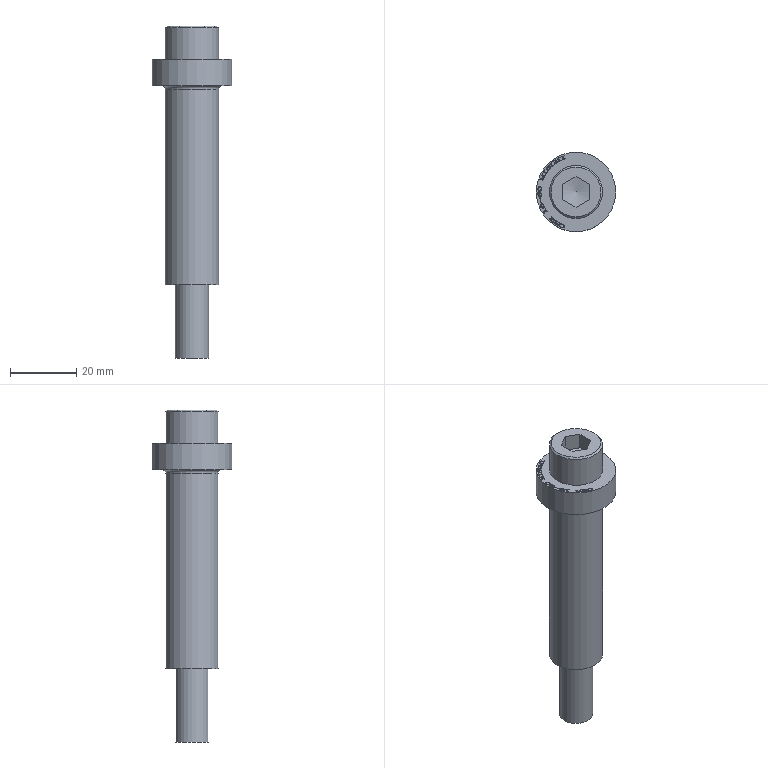Part | STEP file | 1_id2362_x_t | 1 solid | 258 faces | box 24 x 24 x 100 mm | volume 18465 mm3 | other 128 | plane 122 | cylinder 5 | cone 2 | torus 1 | commonest cylinder face diameters 16 x2 10 x1 10.6 x1 24 x1